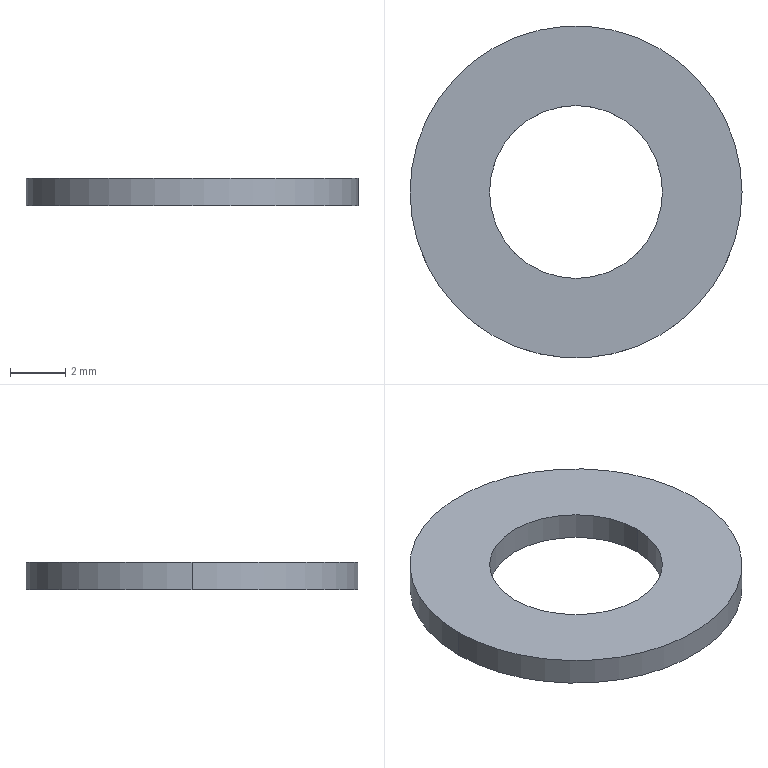Part | SolidWorks | features Extrusion 1 | 1 solid | 6 faces | box 12 x 12 x 1 mm | volume 82.418 mm3 | cylinder 4 | plane 2 | commonest cylinder face diameters 6.25 x2 12 x2
STEP:
#1=CARTESIAN_POINT('',(-0.123,0.,0.03937));
#2=VERTEX_POINT('',#1);
#3=CARTESIAN_POINT('',(0.123,0.,0.03937));
#4=VERTEX_POINT('',#3);
#5=CARTESIAN_POINT('',(0.,0.,0.03937));
#6=DIRECTION('',(0.,0.,1.));
#7=DIRECTION('',(1.,0.,0.));
#8=AXIS2_PLACEMENT_3D('',#5,#6,#7);
#9=CIRCLE('',#8,0.123);
#10=EDGE_CURVE('',#2,#4,#9,.T.);
#11=ORIENTED_EDGE('',*,*,#10,.T.);
#12=CARTESIAN_POINT('',(0.123,0.,0.));
#13=VERTEX_POINT('',#12);
#14=CARTESIAN_POINT('',(0.123,0.,0.03937));
#15=DIRECTION('',(0.,0.,-1.));
#16=VECTOR('',#15,39.37);
#17=LINE('',#14,#16);
#18=EDGE_CURVE('',#4,#13,#17,.T.);
#19=ORIENTED_EDGE('',*,*,#18,.T.);
#20=CARTESIAN_POINT('',(-0.123,0.,0.));
#21=VERTEX_POINT('',#20);
#22=CARTESIAN_POINT('',(0.,0.,0.));
#23=DIRECTION('',(0.,0.,1.));
#24=DIRECTION('',(1.,0.,0.));
#25=AXIS2_PLACEMENT_3D('',#22,#23,#24);
#26=CIRCLE('',#25,0.123);
#27=EDGE_CURVE('',#21,#13,#26,.T.);
#28=ORIENTED_EDGE('',*,*,#27,.F.);
#29=CARTESIAN_POINT('',(-0.123,0.,0.03937));
#30=DIRECTION('',(0.,0.,-1.));
#31=VECTOR('',#30,39.37);
#32=LINE('',#29,#31);
#33=EDGE_CURVE('',#2,#21,#32,.T.);
#34=ORIENTED_EDGE('',*,*,#33,.F.);
#35=EDGE_LOOP('',(#11,#19,#28,#34));
#36=FACE_OUTER_BOUND('',#35,.T.);
#37=CARTESIAN_POINT('',(0.,0.,0.03937));
#38=DIRECTION('',(0.,0.,-1.));
#39=DIRECTION('',(-1.,0.,0.));
#40=AXIS2_PLACEMENT_3D('',#37,#38,#39);
#41=CYLINDRICAL_SURFACE('',#40,0.123);
#42=ADVANCED_FACE('',(#36),#41,.F.);
#43=CARTESIAN_POINT('',(0.2362,0.,0.03937));
#44=VERTEX_POINT('',#43);
#45=CARTESIAN_POINT('',(-0.2362,0.,0.03937));
#46=VERTEX_POINT('',#45);
#47=CARTESIAN_POINT('',(0.,0.,0.03937));
#48=DIRECTION('',(0.,0.,1.));
#49=DIRECTION('',(1.,0.,0.));
#50=AXIS2_PLACEMENT_3D('',#47,#48,#49);
#51=CIRCLE('',#50,0.2362);
#52=EDGE_CURVE('',#44,#46,#51,.T.);
#53=ORIENTED_EDGE('',*,*,#52,.F.);
#54=CARTESIAN_POINT('',(0.2362,0.,0.));
#55=VERTEX_POINT('',#54);
#56=CARTESIAN_POINT('',(0.2362,0.,0.03937));
#57=DIRECTION('',(0.,0.,-1.));
#58=VECTOR('',#57,39.37);
#59=LINE('',#56,#58);
#60=EDGE_CURVE('',#44,#55,#59,.T.);
#61=ORIENTED_EDGE('',*,*,#60,.T.);
#62=CARTESIAN_POINT('',(-0.2362,0.,0.));
#63=VERTEX_POINT('',#62);
#64=CARTESIAN_POINT('',(0.,0.,0.));
#65=DIRECTION('',(0.,0.,1.));
#66=DIRECTION('',(1.,0.,0.));
#67=AXIS2_PLACEMENT_3D('',#64,#65,#66);
#68=CIRCLE('',#67,0.2362);
#69=EDGE_CURVE('',#55,#63,#68,.T.);
#70=ORIENTED_EDGE('',*,*,#69,.T.);
#71=CARTESIAN_POINT('',(-0.2362,0.,0.03937));
#72=DIRECTION('',(0.,0.,-1.));
#73=VECTOR('',#72,39.37);
#74=LINE('',#71,#73);
#75=EDGE_CURVE('',#46,#63,#74,.T.);
#76=ORIENTED_EDGE('',*,*,#75,.F.);
#77=EDGE_LOOP('',(#53,#61,#70,#76));
#78=FACE_OUTER_BOUND('',#77,.T.);
#79=CARTESIAN_POINT('',(0.,0.,0.03937));
#80=DIRECTION('',(0.,0.,-1.));
#81=DIRECTION('',(-1.,0.,0.));
#82=AXIS2_PLACEMENT_3D('',#79,#80,#81);
#83=CYLINDRICAL_SURFACE('',#82,0.2362);
#84=ADVANCED_FACE('',(#78),#83,.T.);
#85=CARTESIAN_POINT('',(0.,0.,0.03937));
#86=DIRECTION('',(0.,0.,1.));
#87=DIRECTION('',(1.,0.,0.));
#88=AXIS2_PLACEMENT_3D('',#85,#86,#87);
#89=CIRCLE('',#88,0.2362);
#90=EDGE_CURVE('',#46,#44,#89,.T.);
#91=ORIENTED_EDGE('',*,*,#90,.T.);
#92=ORIENTED_EDGE('',*,*,#52,.T.);
#93=EDGE_LOOP('',(#91,#92));
#94=FACE_OUTER_BOUND('',#93,.T.);
#95=ORIENTED_EDGE('',*,*,#10,.F.);
#96=CARTESIAN_POINT('',(0.,0.,0.03937));
#97=DIRECTION('',(0.,0.,1.));
#98=DIRECTION('',(1.,0.,0.));
#99=AXIS2_PLACEMENT_3D('',#96,#97,#98);
#100=CIRCLE('',#99,0.123);
#101=EDGE_CURVE('',#4,#2,#100,.T.);
#102=ORIENTED_EDGE('',*,*,#101,.F.);
#103=EDGE_LOOP('',(#95,#102));
#104=FACE_BOUND('',#103,.T.);
#105=CARTESIAN_POINT('',(0.,0.,0.03937));
#106=DIRECTION('',(0.,0.,1.));
#107=DIRECTION('',(1.,0.,0.));
#108=AXIS2_PLACEMENT_3D('',#105,#106,#107);
#109=PLANE('',#108);
#110=ADVANCED_FACE('',(#94,#104),#109,.T.);
#111=CARTESIAN_POINT('',(0.,0.,0.));
#112=DIRECTION('',(0.,0.,1.));
#113=DIRECTION('',(1.,0.,0.));
#114=AXIS2_PLACEMENT_3D('',#111,#112,#113);
#115=CIRCLE('',#114,0.2362);
#116=EDGE_CURVE('',#63,#55,#115,.T.);
#117=ORIENTED_EDGE('',*,*,#116,.F.);
#118=ORIENTED_EDGE('',*,*,#69,.F.);
#119=EDGE_LOOP('',(#117,#118));
#120=FACE_OUTER_BOUND('',#119,.T.);
#121=ORIENTED_EDGE('',*,*,#27,.T.);
#122=CARTESIAN_POINT('',(0.,0.,0.));
#123=DIRECTION('',(0.,0.,1.));
#124=DIRECTION('',(1.,0.,0.));
#125=AXIS2_PLACEMENT_3D('',#122,#123,#124);
#126=CIRCLE('',#125,0.123);
#127=EDGE_CURVE('',#13,#21,#126,.T.);
#128=ORIENTED_EDGE('',*,*,#127,.T.);
#129=EDGE_LOOP('',(#121,#128));
#130=FACE_BOUND('',#129,.T.);
#131=CARTESIAN_POINT('',(0.,0.,0.));
#132=DIRECTION('',(0.,0.,1.));
#133=DIRECTION('',(1.,0.,0.));
#134=AXIS2_PLACEMENT_3D('',#131,#132,#133);
#135=PLANE('',#134);
#136=ADVANCED_FACE('',(#120,#130),#135,.F.);
#137=ORIENTED_EDGE('',*,*,#60,.F.);
#138=ORIENTED_EDGE('',*,*,#90,.F.);
#139=ORIENTED_EDGE('',*,*,#75,.T.);
#140=ORIENTED_EDGE('',*,*,#116,.T.);
#141=EDGE_LOOP('',(#137,#138,#139,#140));
#142=FACE_OUTER_BOUND('',#141,.T.);
#143=CARTESIAN_POINT('',(0.,0.,0.03937));
#144=DIRECTION('',(0.,0.,-1.));
#145=DIRECTION('',(-1.,0.,0.));
#146=AXIS2_PLACEMENT_3D('',#143,#144,#145);
#147=CYLINDRICAL_SURFACE('',#146,0.2362);
#148=ADVANCED_FACE('',(#142),#147,.T.);
#149=ORIENTED_EDGE('',*,*,#18,.F.);
#150=ORIENTED_EDGE('',*,*,#101,.T.);
#151=ORIENTED_EDGE('',*,*,#33,.T.);
#152=ORIENTED_EDGE('',*,*,#127,.F.);
#153=EDGE_LOOP('',(#149,#150,#151,#152));
#154=FACE_OUTER_BOUND('',#153,.T.);
#155=CARTESIAN_POINT('',(0.,0.,0.03937));
#156=DIRECTION('',(0.,0.,-1.));
#157=DIRECTION('',(-1.,0.,0.));
#158=AXIS2_PLACEMENT_3D('',#155,#156,#157);
#159=CYLINDRICAL_SURFACE('',#158,0.123);
#160=ADVANCED_FACE('',(#154),#159,.F.);
#161=CLOSED_SHELL('',(#42,#84,#110,#136,#148,#160));
#162=MANIFOLD_SOLID_BREP('',#161);
#163=CARTESIAN_POINT('',(0.,0.,0.));
#164=DIRECTION('',(0.,0.,1.));
#165=DIRECTION('',(1.,0.,0.));
#166=AXIS2_PLACEMENT_3D('',#163,#164,#165);
#167=(LENGTH_UNIT()NAMED_UNIT(*)SI_UNIT($,.METRE.));
#168=LENGTH_MEASURE_WITH_UNIT(LENGTH_MEASURE(0.0254),#167);
#169=DIMENSIONAL_EXPONENTS(1.,0.,0.,0.,0.,0.,0.);
#170=(CONVERSION_BASED_UNIT('INCH',#168)LENGTH_UNIT()NAMED_UNIT(#169));
#171=UNCERTAINTY_MEASURE_WITH_UNIT(LENGTH_MEASURE(0.00001),#170,'','');
#172=(NAMED_UNIT(*)PLANE_ANGLE_UNIT()SI_UNIT($,.RADIAN.));
#173=(NAMED_UNIT(*)SI_UNIT($,.STERADIAN.)SOLID_ANGLE_UNIT());
#174=(GEOMETRIC_REPRESENTATION_CONTEXT(3)GLOBAL_UNCERTAINTY_ASSIGNED_CONTEXT((#171))GLOBAL_UNIT_ASSIGNED_CONTEXT((#170,#172,#173))REPRESENTATION_CONTEXT('',''));
#175=ADVANCED_BREP_SHAPE_REPRESENTATION('',(#162,#166),#174);